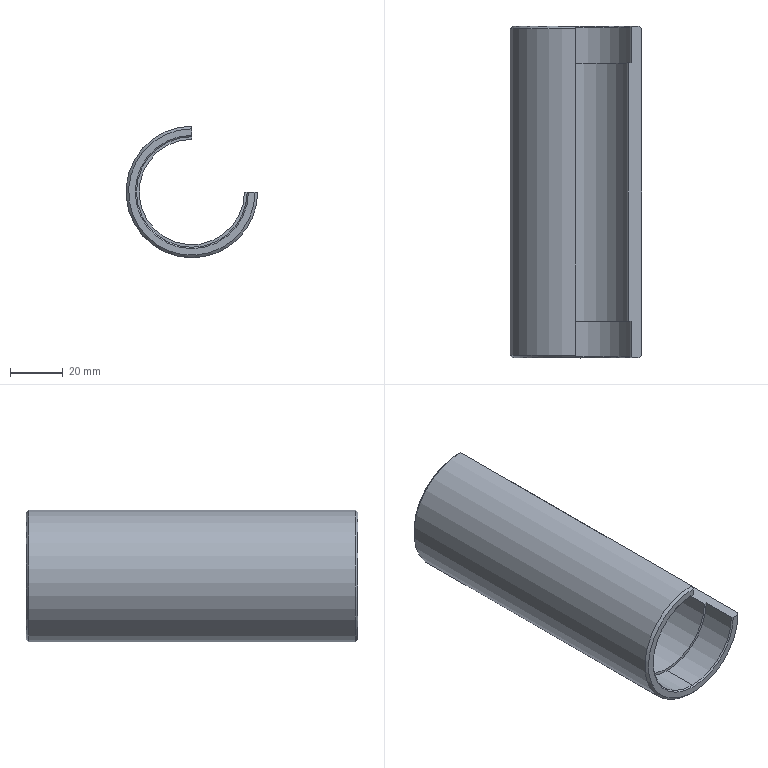Part | STEP file | 1 solid | 18 faces | box 50 x 126 x 50 mm | volume 63952 mm3 | cone 6 | cylinder 6 | plane 6 | commonest cylinder face diameters 42 x3 50 x2 40 x1
STEP:
#1=CARTESIAN_POINT('',(0.,0.,0.));
#2=DIRECTION('',(0.,0.,1.));
#3=DIRECTION('',(1.,0.,0.));
#4=AXIS2_PLACEMENT_3D('',#1,#2,#3);
#5=CARTESIAN_POINT('',(0.,63.,-24.));
#6=VERTEX_POINT('',#5);
#7=CARTESIAN_POINT('',(0.,63.,24.));
#8=VERTEX_POINT('',#7);
#9=CARTESIAN_POINT('',(0.,63.,0.));
#10=DIRECTION('',(0.,1.,0.));
#11=DIRECTION('',(0.,0.,1.));
#12=AXIS2_PLACEMENT_3D('',#9,#10,#11);
#13=CIRCLE('',#12,24.);
#14=CARTESIAN_POINT('',(0.,63.,0.));
#15=DIRECTION('',(0.,-1.,0.));
#16=DIRECTION('',(0.,0.,-1.));
#17=AXIS2_PLACEMENT_3D('',#14,#15,#16);
#18=CONICAL_SURFACE('',#17,24.,0.7854);
#19=CARTESIAN_POINT('',(9.425,0.));
#20=DIRECTION('',(-1.,0.));
#21=VECTOR('',#20,1.);
#22=LINE('',#19,#21);
#23=(GEOMETRIC_REPRESENTATION_CONTEXT(2)PARAMETRIC_REPRESENTATION_CONTEXT()REPRESENTATION_CONTEXT('',''));
#24=DEFINITIONAL_REPRESENTATION('',(#22),#23);
#25=PCURVE('',#18,#24);
#26=CARTESIAN_POINT('',(0.,63.,0.));
#27=DIRECTION('',(0.,1.,0.));
#28=DIRECTION('',(0.,0.,1.));
#29=AXIS2_PLACEMENT_3D('',#26,#27,#28);
#30=PLANE('',#29);
#31=CARTESIAN_POINT('',(0.,0.));
#32=DIRECTION('',(1.,0.));
#33=AXIS2_PLACEMENT_2D('',#31,#32);
#34=CIRCLE('',#33,24.);
#35=(GEOMETRIC_REPRESENTATION_CONTEXT(2)PARAMETRIC_REPRESENTATION_CONTEXT()REPRESENTATION_CONTEXT('',''));
#36=DEFINITIONAL_REPRESENTATION('',(#34),#35);
#37=PCURVE('',#30,#36);
#38=SURFACE_CURVE('',#13,(#25,#37),.PCURVE_S1.);
#39=EDGE_CURVE('',#6,#8,#38,.T.);
#40=ORIENTED_EDGE('',*,*,#39,.F.);
#41=CARTESIAN_POINT('',(0.,62.,-25.));
#42=VERTEX_POINT('',#41);
#43=CARTESIAN_POINT('',(0.,63.,-24.));
#44=DIRECTION('',(0.,-0.7071,-0.7071));
#45=VECTOR('',#44,1.);
#46=LINE('',#43,#45);
#47=CARTESIAN_POINT('',(6.283,0.));
#48=DIRECTION('',(0.,1.));
#49=VECTOR('',#48,1.);
#50=LINE('',#47,#49);
#51=(GEOMETRIC_REPRESENTATION_CONTEXT(2)PARAMETRIC_REPRESENTATION_CONTEXT()REPRESENTATION_CONTEXT('',''));
#52=DEFINITIONAL_REPRESENTATION('',(#50),#51);
#53=PCURVE('',#18,#52);
#54=CARTESIAN_POINT('',(0.,63.,0.));
#55=DIRECTION('',(0.,-1.,0.));
#56=DIRECTION('',(0.,0.,-1.));
#57=AXIS2_PLACEMENT_3D('',#54,#55,#56);
#58=CONICAL_SURFACE('',#57,24.,0.7854);
#59=CARTESIAN_POINT('',(0.,0.));
#60=DIRECTION('',(0.,1.));
#61=VECTOR('',#60,1.);
#62=LINE('',#59,#61);
#63=(GEOMETRIC_REPRESENTATION_CONTEXT(2)PARAMETRIC_REPRESENTATION_CONTEXT()REPRESENTATION_CONTEXT('',''));
#64=DEFINITIONAL_REPRESENTATION('',(#62),#63);
#65=PCURVE('',#58,#64);
#66=SURFACE_CURVE('',#46,(#53,#65),.PCURVE_S1.);
#67=EDGE_CURVE('',#6,#42,#66,.T.);
#68=ORIENTED_EDGE('',*,*,#67,.T.);
#69=CARTESIAN_POINT('',(0.,62.,25.));
#70=VERTEX_POINT('',#69);
#71=CARTESIAN_POINT('',(0.,62.,0.));
#72=DIRECTION('',(0.,-1.,0.));
#73=DIRECTION('',(0.,0.,1.));
#74=AXIS2_PLACEMENT_3D('',#71,#72,#73);
#75=CIRCLE('',#74,25.);
#76=CARTESIAN_POINT('',(3.142,1.));
#77=DIRECTION('',(1.,0.));
#78=VECTOR('',#77,1.);
#79=LINE('',#76,#78);
#80=(GEOMETRIC_REPRESENTATION_CONTEXT(2)PARAMETRIC_REPRESENTATION_CONTEXT()REPRESENTATION_CONTEXT('',''));
#81=DEFINITIONAL_REPRESENTATION('',(#79),#80);
#82=PCURVE('',#18,#81);
#83=CARTESIAN_POINT('',(0.,63.,0.));
#84=DIRECTION('',(0.,-1.,0.));
#85=DIRECTION('',(0.,0.,-1.));
#86=AXIS2_PLACEMENT_3D('',#83,#84,#85);
#87=CYLINDRICAL_SURFACE('',#86,25.);
#88=CARTESIAN_POINT('',(3.142,1.));
#89=DIRECTION('',(1.,0.));
#90=VECTOR('',#89,1.);
#91=LINE('',#88,#90);
#92=(GEOMETRIC_REPRESENTATION_CONTEXT(2)PARAMETRIC_REPRESENTATION_CONTEXT()REPRESENTATION_CONTEXT('',''));
#93=DEFINITIONAL_REPRESENTATION('',(#91),#92);
#94=PCURVE('',#87,#93);
#95=SURFACE_CURVE('',#75,(#82,#94),.PCURVE_S1.);
#96=EDGE_CURVE('',#70,#42,#95,.T.);
#97=ORIENTED_EDGE('',*,*,#96,.F.);
#98=CARTESIAN_POINT('',(0.,87.,0.));
#99=DIRECTION('',(0.,-0.7071,0.7071));
#100=VECTOR('',#99,1.);
#101=LINE('',#98,#100);
#102=CARTESIAN_POINT('',(3.142,-24.));
#103=DIRECTION('',(0.,1.));
#104=VECTOR('',#103,1.);
#105=LINE('',#102,#104);
#106=(GEOMETRIC_REPRESENTATION_CONTEXT(2)PARAMETRIC_REPRESENTATION_CONTEXT()REPRESENTATION_CONTEXT('',''));
#107=DEFINITIONAL_REPRESENTATION('',(#105),#106);
#108=PCURVE('',#18,#107);
#109=CARTESIAN_POINT('',(0.,95.,25.));
#110=DIRECTION('',(-1.,0.,0.));
#111=DIRECTION('',(0.,0.,1.));
#112=AXIS2_PLACEMENT_3D('',#109,#110,#111);
#113=PLANE('',#112);
#114=CARTESIAN_POINT('',(-25.,-8.));
#115=DIRECTION('',(0.7071,-0.7071));
#116=VECTOR('',#115,1.);
#117=LINE('',#114,#116);
#118=(GEOMETRIC_REPRESENTATION_CONTEXT(2)PARAMETRIC_REPRESENTATION_CONTEXT()REPRESENTATION_CONTEXT('',''));
#119=DEFINITIONAL_REPRESENTATION('',(#117),#118);
#120=PCURVE('',#113,#119);
#121=SURFACE_CURVE('',#101,(#108,#120),.PCURVE_S1.);
#122=EDGE_CURVE('',#8,#70,#121,.T.);
#123=ORIENTED_EDGE('',*,*,#122,.F.);
#124=EDGE_LOOP('',(#40,#68,#97,#123));
#125=FACE_BOUND('',#124,.T.);
#126=ADVANCED_FACE('',(#125),#18,.T.);
#127=CARTESIAN_POINT('',(21.,-62.5,0.));
#128=VERTEX_POINT('',#127);
#129=CARTESIAN_POINT('',(21.5,-63.,0.));
#130=VERTEX_POINT('',#129);
#131=CARTESIAN_POINT('',(0.,-41.5,0.));
#132=DIRECTION('',(0.7071,-0.7071,0.));
#133=VECTOR('',#132,1.);
#134=LINE('',#131,#133);
#135=CARTESIAN_POINT('',(0.,-63.,0.));
#136=DIRECTION('',(0.,-1.,0.));
#137=DIRECTION('',(0.,0.,-1.));
#138=AXIS2_PLACEMENT_3D('',#135,#136,#137);
#139=CONICAL_SURFACE('',#138,21.5,0.7854);
#140=CARTESIAN_POINT('',(1.571,-21.5));
#141=DIRECTION('',(0.,1.));
#142=VECTOR('',#141,1.);
#143=LINE('',#140,#142);
#144=(GEOMETRIC_REPRESENTATION_CONTEXT(2)PARAMETRIC_REPRESENTATION_CONTEXT()REPRESENTATION_CONTEXT('',''));
#145=DEFINITIONAL_REPRESENTATION('',(#143),#144);
#146=PCURVE('',#139,#145);
#147=CARTESIAN_POINT('',(0.,95.,0.));
#148=DIRECTION('',(0.,0.,-1.));
#149=DIRECTION('',(-1.,0.,0.));
#150=AXIS2_PLACEMENT_3D('',#147,#148,#149);
#151=PLANE('',#150);
#152=CARTESIAN_POINT('',(0.,-136.5));
#153=DIRECTION('',(-0.7071,-0.7071));
#154=VECTOR('',#153,1.);
#155=LINE('',#152,#154);
#156=(GEOMETRIC_REPRESENTATION_CONTEXT(2)PARAMETRIC_REPRESENTATION_CONTEXT()REPRESENTATION_CONTEXT('',''));
#157=DEFINITIONAL_REPRESENTATION('',(#155),#156);
#158=PCURVE('',#151,#157);
#159=SURFACE_CURVE('',#134,(#146,#158),.PCURVE_S1.);
#160=EDGE_CURVE('',#128,#130,#159,.T.);
#161=ORIENTED_EDGE('',*,*,#160,.T.);
#162=CARTESIAN_POINT('',(0.,-63.,-21.5));
#163=VERTEX_POINT('',#162);
#164=CARTESIAN_POINT('',(0.,-63.,0.));
#165=DIRECTION('',(0.,1.,0.));
#166=DIRECTION('',(0.,0.,1.));
#167=AXIS2_PLACEMENT_3D('',#164,#165,#166);
#168=CIRCLE('',#167,21.5);
#169=CARTESIAN_POINT('',(3.142,0.));
#170=DIRECTION('',(-1.,0.));
#171=VECTOR('',#170,1.);
#172=LINE('',#169,#171);
#173=(GEOMETRIC_REPRESENTATION_CONTEXT(2)PARAMETRIC_REPRESENTATION_CONTEXT()REPRESENTATION_CONTEXT('',''));
#174=DEFINITIONAL_REPRESENTATION('',(#172),#173);
#175=PCURVE('',#139,#174);
#176=CARTESIAN_POINT('',(0.,-63.,0.));
#177=DIRECTION('',(0.,1.,0.));
#178=DIRECTION('',(0.,0.,1.));
#179=AXIS2_PLACEMENT_3D('',#176,#177,#178);
#180=PLANE('',#179);
#181=CARTESIAN_POINT('',(0.,0.));
#182=DIRECTION('',(1.,0.));
#183=AXIS2_PLACEMENT_2D('',#181,#182);
#184=CIRCLE('',#183,21.5);
#185=(GEOMETRIC_REPRESENTATION_CONTEXT(2)PARAMETRIC_REPRESENTATION_CONTEXT()REPRESENTATION_CONTEXT('',''));
#186=DEFINITIONAL_REPRESENTATION('',(#184),#185);
#187=PCURVE('',#180,#186);
#188=SURFACE_CURVE('',#168,(#175,#187),.PCURVE_S1.);
#189=EDGE_CURVE('',#130,#163,#188,.T.);
#190=ORIENTED_EDGE('',*,*,#189,.T.);
#191=CARTESIAN_POINT('',(0.,-62.5,-21.));
#192=VERTEX_POINT('',#191);
#193=CARTESIAN_POINT('',(0.,-63.,-21.5));
#194=DIRECTION('',(0.,-0.7071,-0.7071));
#195=VECTOR('',#194,1.);
#196=LINE('',#193,#195);
#197=CARTESIAN_POINT('',(0.,0.));
#198=DIRECTION('',(0.,1.));
#199=VECTOR('',#198,1.);
#200=LINE('',#197,#199);
#201=(GEOMETRIC_REPRESENTATION_CONTEXT(2)PARAMETRIC_REPRESENTATION_CONTEXT()REPRESENTATION_CONTEXT('',''));
#202=DEFINITIONAL_REPRESENTATION('',(#200),#201);
#203=PCURVE('',#139,#202);
#204=CARTESIAN_POINT('',(0.,-63.,0.));
#205=DIRECTION('',(0.,-1.,0.));
#206=DIRECTION('',(0.,0.,-1.));
#207=AXIS2_PLACEMENT_3D('',#204,#205,#206);
#208=CONICAL_SURFACE('',#207,21.5,0.7854);
#209=CARTESIAN_POINT('',(6.283,0.));
#210=DIRECTION('',(0.,1.));
#211=VECTOR('',#210,1.);
#212=LINE('',#209,#211);
#213=(GEOMETRIC_REPRESENTATION_CONTEXT(2)PARAMETRIC_REPRESENTATION_CONTEXT()REPRESENTATION_CONTEXT('',''));
#214=DEFINITIONAL_REPRESENTATION('',(#212),#213);
#215=PCURVE('',#208,#214);
#216=SURFACE_CURVE('',#196,(#203,#215),.PCURVE_S1.);
#217=EDGE_CURVE('',#192,#163,#216,.T.);
#218=ORIENTED_EDGE('',*,*,#217,.F.);
#219=CARTESIAN_POINT('',(0.,-62.5,0.));
#220=DIRECTION('',(0.,-1.,0.));
#221=DIRECTION('',(0.,0.,1.));
#222=AXIS2_PLACEMENT_3D('',#219,#220,#221);
#223=CIRCLE('',#222,21.);
#224=CARTESIAN_POINT('',(-3.142,-0.5));
#225=DIRECTION('',(1.,0.));
#226=VECTOR('',#225,1.);
#227=LINE('',#224,#226);
#228=(GEOMETRIC_REPRESENTATION_CONTEXT(2)PARAMETRIC_REPRESENTATION_CONTEXT()REPRESENTATION_CONTEXT('',''));
#229=DEFINITIONAL_REPRESENTATION('',(#227),#228);
#230=PCURVE('',#139,#229);
#231=CARTESIAN_POINT('',(0.,-49.,0.));
#232=DIRECTION('',(0.,-1.,0.));
#233=DIRECTION('',(0.,0.,-1.));
#234=AXIS2_PLACEMENT_3D('',#231,#232,#233);
#235=CYLINDRICAL_SURFACE('',#234,21.);
#236=CARTESIAN_POINT('',(-3.142,13.5));
#237=DIRECTION('',(1.,0.));
#238=VECTOR('',#237,1.);
#239=LINE('',#236,#238);
#240=(GEOMETRIC_REPRESENTATION_CONTEXT(2)PARAMETRIC_REPRESENTATION_CONTEXT()REPRESENTATION_CONTEXT('',''));
#241=DEFINITIONAL_REPRESENTATION('',(#239),#240);
#242=PCURVE('',#235,#241);
#243=SURFACE_CURVE('',#223,(#230,#242),.PCURVE_S1.);
#244=EDGE_CURVE('',#192,#128,#243,.T.);
#245=ORIENTED_EDGE('',*,*,#244,.T.);
#246=EDGE_LOOP('',(#161,#190,#218,#245));
#247=FACE_BOUND('',#246,.F.);
#248=ADVANCED_FACE('',(#247),#139,.F.);
#249=CARTESIAN_POINT('',(21.,-49.,0.));
#250=VERTEX_POINT('',#249);
#251=CARTESIAN_POINT('',(21.,-49.,0.));
#252=DIRECTION('',(0.,-1.,0.));
#253=VECTOR('',#252,1.);
#254=LINE('',#251,#253);
#255=CARTESIAN_POINT('',(1.571,0.));
#256=DIRECTION('',(0.,1.));
#257=VECTOR('',#256,1.);
#258=LINE('',#255,#257);
#259=(GEOMETRIC_REPRESENTATION_CONTEXT(2)PARAMETRIC_REPRESENTATION_CONTEXT()REPRESENTATION_CONTEXT('',''));
#260=DEFINITIONAL_REPRESENTATION('',(#258),#259);
#261=PCURVE('',#235,#260);
#262=CARTESIAN_POINT('',(-21.,-144.));
#263=DIRECTION('',(0.,-1.));
#264=VECTOR('',#263,1.);
#265=LINE('',#262,#264);
#266=(GEOMETRIC_REPRESENTATION_CONTEXT(2)PARAMETRIC_REPRESENTATION_CONTEXT()REPRESENTATION_CONTEXT('',''));
#267=DEFINITIONAL_REPRESENTATION('',(#265),#266);
#268=PCURVE('',#151,#267);
#269=SURFACE_CURVE('',#254,(#261,#268),.PCURVE_S1.);
#270=EDGE_CURVE('',#250,#128,#269,.T.);
#271=ORIENTED_EDGE('',*,*,#270,.T.);
#272=ORIENTED_EDGE('',*,*,#244,.F.);
#273=CARTESIAN_POINT('',(0.,-49.,-21.));
#274=VERTEX_POINT('',#273);
#275=CARTESIAN_POINT('',(0.,-49.,-21.));
#276=DIRECTION('',(0.,-1.,0.));
#277=VECTOR('',#276,1.);
#278=LINE('',#275,#277);
#279=CARTESIAN_POINT('',(0.,0.));
#280=DIRECTION('',(0.,1.));
#281=VECTOR('',#280,1.);
#282=LINE('',#279,#281);
#283=(GEOMETRIC_REPRESENTATION_CONTEXT(2)PARAMETRIC_REPRESENTATION_CONTEXT()REPRESENTATION_CONTEXT('',''));
#284=DEFINITIONAL_REPRESENTATION('',(#282),#283);
#285=PCURVE('',#235,#284);
#286=CARTESIAN_POINT('',(0.,-49.,0.));
#287=DIRECTION('',(0.,-1.,0.));
#288=DIRECTION('',(0.,0.,-1.));
#289=AXIS2_PLACEMENT_3D('',#286,#287,#288);
#290=CYLINDRICAL_SURFACE('',#289,21.);
#291=CARTESIAN_POINT('',(6.283,0.));
#292=DIRECTION('',(0.,1.));
#293=VECTOR('',#292,1.);
#294=LINE('',#291,#293);
#295=(GEOMETRIC_REPRESENTATION_CONTEXT(2)PARAMETRIC_REPRESENTATION_CONTEXT()REPRESENTATION_CONTEXT('',''));
#296=DEFINITIONAL_REPRESENTATION('',(#294),#295);
#297=PCURVE('',#290,#296);
#298=SURFACE_CURVE('',#278,(#285,#297),.PCURVE_S1.);
#299=EDGE_CURVE('',#274,#192,#298,.T.);
#300=ORIENTED_EDGE('',*,*,#299,.F.);
#301=CARTESIAN_POINT('',(0.,-49.,0.));
#302=DIRECTION('',(0.,1.,0.));
#303=DIRECTION('',(0.,0.,1.));
#304=AXIS2_PLACEMENT_3D('',#301,#302,#303);
#305=CIRCLE('',#304,21.);
#306=CARTESIAN_POINT('',(3.142,0.));
#307=DIRECTION('',(-1.,0.));
#308=VECTOR('',#307,1.);
#309=LINE('',#306,#308);
#310=(GEOMETRIC_REPRESENTATION_CONTEXT(2)PARAMETRIC_REPRESENTATION_CONTEXT()REPRESENTATION_CONTEXT('',''));
#311=DEFINITIONAL_REPRESENTATION('',(#309),#310);
#312=PCURVE('',#235,#311);
#313=CARTESIAN_POINT('',(0.,-49.,0.));
#314=DIRECTION('',(0.,-1.,0.));
#315=DIRECTION('',(0.,0.,1.));
#316=AXIS2_PLACEMENT_3D('',#313,#314,#315);
#317=PLANE('',#316);
#318=CARTESIAN_POINT('',(21.,0.));
#319=CARTESIAN_POINT('',(21.,-36.373));
#320=CARTESIAN_POINT('',(-10.5,-18.187));
#321=CARTESIAN_POINT('',(-42.,0.));
#322=CARTESIAN_POINT('',(-10.5,18.187));
#323=CARTESIAN_POINT('',(21.,36.373));
#324=CARTESIAN_POINT('',(21.,0.));
#325=(BOUNDED_CURVE()B_SPLINE_CURVE(2,(#318,#319,#320,#321,#322,#323,#324),.UNSPECIFIED.,.T.,.F.)B_SPLINE_CURVE_WITH_KNOTS((1,2,2,2,2,1),(-2.094,0.,2.094,4.189,6.283,8.378),.UNSPECIFIED.)CURVE()GEOMETRIC_REPRESENTATION_ITEM()RATIONAL_B_SPLINE_CURVE((1.,0.5,1.,0.5,1.,0.5,1.))REPRESENTATION_ITEM(''));
#326=(GEOMETRIC_REPRESENTATION_CONTEXT(2)PARAMETRIC_REPRESENTATION_CONTEXT()REPRESENTATION_CONTEXT('',''));
#327=DEFINITIONAL_REPRESENTATION('',(#325),#326);
#328=PCURVE('',#317,#327);
#329=SURFACE_CURVE('',#305,(#312,#328),.PCURVE_S1.);
#330=EDGE_CURVE('',#250,#274,#329,.T.);
#331=ORIENTED_EDGE('',*,*,#330,.F.);
#332=EDGE_LOOP('',(#271,#272,#300,#331));
#333=FACE_BOUND('',#332,.F.);
#334=ADVANCED_FACE('',(#333),#235,.F.);
#335=ORIENTED_EDGE('',*,*,#96,.T.);
#336=CARTESIAN_POINT('',(0.,-62.,-25.));
#337=VERTEX_POINT('',#336);
#338=CARTESIAN_POINT('',(0.,63.,-25.));
#339=DIRECTION('',(0.,-1.,0.));
#340=VECTOR('',#339,1.);
#341=LINE('',#338,#340);
#342=CARTESIAN_POINT('',(6.283,0.));
#343=DIRECTION('',(0.,1.));
#344=VECTOR('',#343,1.);
#345=LINE('',#342,#344);
#346=(GEOMETRIC_REPRESENTATION_CONTEXT(2)PARAMETRIC_REPRESENTATION_CONTEXT()REPRESENTATION_CONTEXT('',''));
#347=DEFINITIONAL_REPRESENTATION('',(#345),#346);
#348=PCURVE('',#87,#347);
#349=CARTESIAN_POINT('',(0.,63.,0.));
#350=DIRECTION('',(0.,-1.,0.));
#351=DIRECTION('',(0.,0.,-1.));
#352=AXIS2_PLACEMENT_3D('',#349,#350,#351);
#353=CYLINDRICAL_SURFACE('',#352,25.);
#354=CARTESIAN_POINT('',(0.,0.));
#355=DIRECTION('',(0.,1.));
#356=VECTOR('',#355,1.);
#357=LINE('',#354,#356);
#358=(GEOMETRIC_REPRESENTATION_CONTEXT(2)PARAMETRIC_REPRESENTATION_CONTEXT()REPRESENTATION_CONTEXT('',''));
#359=DEFINITIONAL_REPRESENTATION('',(#357),#358);
#360=PCURVE('',#353,#359);
#361=SURFACE_CURVE('',#341,(#348,#360),.PCURVE_S1.);
#362=EDGE_CURVE('',#42,#337,#361,.T.);
#363=ORIENTED_EDGE('',*,*,#362,.T.);
#364=CARTESIAN_POINT('',(0.,-62.,25.));
#365=VERTEX_POINT('',#364);
#366=CARTESIAN_POINT('',(0.,-62.,0.));
#367=DIRECTION('',(0.,1.,0.));
#368=DIRECTION('',(0.,0.,1.));
#369=AXIS2_PLACEMENT_3D('',#366,#367,#368);
#370=CIRCLE('',#369,25.);
#371=CARTESIAN_POINT('',(9.425,125.));
#372=DIRECTION('',(-1.,0.));
#373=VECTOR('',#372,1.);
#374=LINE('',#371,#373);
#375=(GEOMETRIC_REPRESENTATION_CONTEXT(2)PARAMETRIC_REPRESENTATION_CONTEXT()REPRESENTATION_CONTEXT('',''));
#376=DEFINITIONAL_REPRESENTATION('',(#374),#375);
#377=PCURVE('',#87,#376);
#378=CARTESIAN_POINT('',(0.,-62.,0.));
#379=DIRECTION('',(0.,1.,0.));
#380=DIRECTION('',(0.,0.,1.));
#381=AXIS2_PLACEMENT_3D('',#378,#379,#380);
#382=CONICAL_SURFACE('',#381,25.,0.7854);
#383=CARTESIAN_POINT('',(0.,0.));
#384=DIRECTION('',(1.,0.));
#385=VECTOR('',#384,1.);
#386=LINE('',#383,#385);
#387=(GEOMETRIC_REPRESENTATION_CONTEXT(2)PARAMETRIC_REPRESENTATION_CONTEXT()REPRESENTATION_CONTEXT('',''));
#388=DEFINITIONAL_REPRESENTATION('',(#386),#387);
#389=PCURVE('',#382,#388);
#390=SURFACE_CURVE('',#370,(#377,#389),.PCURVE_S1.);
#391=EDGE_CURVE('',#337,#365,#390,.T.);
#392=ORIENTED_EDGE('',*,*,#391,.T.);
#393=CARTESIAN_POINT('',(0.,95.,25.));
#394=DIRECTION('',(0.,-1.,0.));
#395=VECTOR('',#394,1.);
#396=LINE('',#393,#395);
#397=CARTESIAN_POINT('',(3.142,-32.));
#398=DIRECTION('',(0.,1.));
#399=VECTOR('',#398,1.);
#400=LINE('',#397,#399);
#401=(GEOMETRIC_REPRESENTATION_CONTEXT(2)PARAMETRIC_REPRESENTATION_CONTEXT()REPRESENTATION_CONTEXT('',''));
#402=DEFINITIONAL_REPRESENTATION('',(#400),#401);
#403=PCURVE('',#87,#402);
#404=CARTESIAN_POINT('',(0.,0.));
#405=DIRECTION('',(0.,-1.));
#406=VECTOR('',#405,1.);
#407=LINE('',#404,#406);
#408=(GEOMETRIC_REPRESENTATION_CONTEXT(2)PARAMETRIC_REPRESENTATION_CONTEXT()REPRESENTATION_CONTEXT('',''));
#409=DEFINITIONAL_REPRESENTATION('',(#407),#408);
#410=PCURVE('',#113,#409);
#411=SURFACE_CURVE('',#396,(#403,#410),.PCURVE_S1.);
#412=EDGE_CURVE('',#70,#365,#411,.T.);
#413=ORIENTED_EDGE('',*,*,#412,.F.);
#414=EDGE_LOOP('',(#335,#363,#392,#413));
#415=FACE_BOUND('',#414,.T.);
#416=ADVANCED_FACE('',(#415),#87,.T.);
#417=ORIENTED_EDGE('',*,*,#362,.F.);
#418=CARTESIAN_POINT('',(25.,62.,0.));
#419=VERTEX_POINT('',#418);
#420=CARTESIAN_POINT('',(0.,62.,0.));
#421=DIRECTION('',(0.,-1.,0.));
#422=DIRECTION('',(0.,0.,1.));
#423=AXIS2_PLACEMENT_3D('',#420,#421,#422);
#424=CIRCLE('',#423,25.);
#425=CARTESIAN_POINT('',(-3.142,1.));
#426=DIRECTION('',(1.,0.));
#427=VECTOR('',#426,1.);
#428=LINE('',#425,#427);
#429=(GEOMETRIC_REPRESENTATION_CONTEXT(2)PARAMETRIC_REPRESENTATION_CONTEXT()REPRESENTATION_CONTEXT('',''));
#430=DEFINITIONAL_REPRESENTATION('',(#428),#429);
#431=PCURVE('',#353,#430);
#432=CARTESIAN_POINT('',(-3.142,1.));
#433=DIRECTION('',(1.,0.));
#434=VECTOR('',#433,1.);
#435=LINE('',#432,#434);
#436=(GEOMETRIC_REPRESENTATION_CONTEXT(2)PARAMETRIC_REPRESENTATION_CONTEXT()REPRESENTATION_CONTEXT('',''));
#437=DEFINITIONAL_REPRESENTATION('',(#435),#436);
#438=PCURVE('',#58,#437);
#439=SURFACE_CURVE('',#424,(#431,#438),.PCURVE_S1.);
#440=EDGE_CURVE('',#42,#419,#439,.T.);
#441=ORIENTED_EDGE('',*,*,#440,.T.);
#442=CARTESIAN_POINT('',(25.,-62.,0.));
#443=VERTEX_POINT('',#442);
#444=CARTESIAN_POINT('',(25.,63.,0.));
#445=DIRECTION('',(0.,-1.,0.));
#446=VECTOR('',#445,1.);
#447=LINE('',#444,#446);
#448=CARTESIAN_POINT('',(1.571,0.));
#449=DIRECTION('',(0.,1.));
#450=VECTOR('',#449,1.);
#451=LINE('',#448,#450);
#452=(GEOMETRIC_REPRESENTATION_CONTEXT(2)PARAMETRIC_REPRESENTATION_CONTEXT()REPRESENTATION_CONTEXT('',''));
#453=DEFINITIONAL_REPRESENTATION('',(#451),#452);
#454=PCURVE('',#353,#453);
#455=CARTESIAN_POINT('',(-25.,-32.));
#456=DIRECTION('',(0.,-1.));
#457=VECTOR('',#456,1.);
#458=LINE('',#455,#457);
#459=(GEOMETRIC_REPRESENTATION_CONTEXT(2)PARAMETRIC_REPRESENTATION_CONTEXT()REPRESENTATION_CONTEXT('',''));
#460=DEFINITIONAL_REPRESENTATION('',(#458),#459);
#461=PCURVE('',#151,#460);
#462=SURFACE_CURVE('',#447,(#454,#461),.PCURVE_S1.);
#463=EDGE_CURVE('',#419,#443,#462,.T.);
#464=ORIENTED_EDGE('',*,*,#463,.T.);
#465=CARTESIAN_POINT('',(0.,-62.,0.));
#466=DIRECTION('',(0.,1.,0.));
#467=DIRECTION('',(0.,0.,1.));
#468=AXIS2_PLACEMENT_3D('',#465,#466,#467);
#469=CIRCLE('',#468,25.);
#470=CARTESIAN_POINT('',(3.142,125.));
#471=DIRECTION('',(-1.,0.));
#472=VECTOR('',#471,1.);
#473=LINE('',#470,#472);
#474=(GEOMETRIC_REPRESENTATION_CONTEXT(2)PARAMETRIC_REPRESENTATION_CONTEXT()REPRESENTATION_CONTEXT('',''));
#475=DEFINITIONAL_REPRESENTATION('',(#473),#474);
#476=PCURVE('',#353,#475);
#477=CARTESIAN_POINT('',(0.,0.));
#478=DIRECTION('',(1.,0.));
#479=VECTOR('',#478,1.);
#480=LINE('',#477,#479);
#481=(GEOMETRIC_REPRESENTATION_CONTEXT(2)PARAMETRIC_REPRESENTATION_CONTEXT()REPRESENTATION_CONTEXT('',''));
#482=DEFINITIONAL_REPRESENTATION('',(#480),#481);
#483=PCURVE('',#382,#482);
#484=SURFACE_CURVE('',#469,(#476,#483),.PCURVE_S1.);
#485=EDGE_CURVE('',#443,#337,#484,.T.);
#486=ORIENTED_EDGE('',*,*,#485,.T.);
#487=EDGE_LOOP('',(#417,#441,#464,#486));
#488=FACE_BOUND('',#487,.T.);
#489=ADVANCED_FACE('',(#488),#353,.T.);
#490=ORIENTED_EDGE('',*,*,#189,.T.);
#491=CARTESIAN_POINT('',(0.,-63.,21.5));
#492=VERTEX_POINT('',#491);
#493=CARTESIAN_POINT('',(0.,-63.,0.));
#494=DIRECTION('',(0.,1.,0.));
#495=DIRECTION('',(0.,0.,1.));
#496=AXIS2_PLACEMENT_3D('',#493,#494,#495);
#497=CIRCLE('',#496,21.5);
#498=CARTESIAN_POINT('',(0.,0.));
#499=DIRECTION('',(1.,0.));
#500=AXIS2_PLACEMENT_2D('',#498,#499);
#501=CIRCLE('',#500,21.5);
#502=(GEOMETRIC_REPRESENTATION_CONTEXT(2)PARAMETRIC_REPRESENTATION_CONTEXT()REPRESENTATION_CONTEXT('',''));
#503=DEFINITIONAL_REPRESENTATION('',(#501),#502);
#504=PCURVE('',#180,#503);
#505=CARTESIAN_POINT('',(9.425,0.));
#506=DIRECTION('',(-1.,0.));
#507=VECTOR('',#506,1.);
#508=LINE('',#505,#507);
#509=(GEOMETRIC_REPRESENTATION_CONTEXT(2)PARAMETRIC_REPRESENTATION_CONTEXT()REPRESENTATION_CONTEXT('',''));
#510=DEFINITIONAL_REPRESENTATION('',(#508),#509);
#511=PCURVE('',#208,#510);
#512=SURFACE_CURVE('',#497,(#504,#511),.PCURVE_S1.);
#513=EDGE_CURVE('',#163,#492,#512,.T.);
#514=ORIENTED_EDGE('',*,*,#513,.T.);
#515=CARTESIAN_POINT('',(0.,-63.,24.));
#516=VERTEX_POINT('',#515);
#517=CARTESIAN_POINT('',(0.,-63.,0.));
#518=DIRECTION('',(0.,0.,1.));
#519=VECTOR('',#518,1.);
#520=LINE('',#517,#519);
#521=CARTESIAN_POINT('',(0.,0.));
#522=DIRECTION('',(1.,0.));
#523=VECTOR('',#522,1.);
#524=LINE('',#521,#523);
#525=(GEOMETRIC_REPRESENTATION_CONTEXT(2)PARAMETRIC_REPRESENTATION_CONTEXT()REPRESENTATION_CONTEXT('',''));
#526=DEFINITIONAL_REPRESENTATION('',(#524),#525);
#527=PCURVE('',#180,#526);
#528=CARTESIAN_POINT('',(-25.,-158.));
#529=DIRECTION('',(1.,0.));
#530=VECTOR('',#529,1.);
#531=LINE('',#528,#530);
#532=(GEOMETRIC_REPRESENTATION_CONTEXT(2)PARAMETRIC_REPRESENTATION_CONTEXT()REPRESENTATION_CONTEXT('',''));
#533=DEFINITIONAL_REPRESENTATION('',(#531),#532);
#534=PCURVE('',#113,#533);
#535=SURFACE_CURVE('',#520,(#527,#534),.PCURVE_S1.);
#536=EDGE_CURVE('',#492,#516,#535,.T.);
#537=ORIENTED_EDGE('',*,*,#536,.T.);
#538=CARTESIAN_POINT('',(24.,-63.,0.));
#539=VERTEX_POINT('',#538);
#540=CARTESIAN_POINT('',(0.,-63.,0.));
#541=DIRECTION('',(0.,-1.,0.));
#542=DIRECTION('',(0.,0.,1.));
#543=AXIS2_PLACEMENT_3D('',#540,#541,#542);
#544=CIRCLE('',#543,24.);
#545=CARTESIAN_POINT('',(24.,0.));
#546=CARTESIAN_POINT('',(24.,-41.569));
#547=CARTESIAN_POINT('',(-12.,-20.785));
#548=CARTESIAN_POINT('',(-48.,0.));
#549=CARTESIAN_POINT('',(-12.,20.785));
#550=CARTESIAN_POINT('',(24.,41.569));
#551=CARTESIAN_POINT('',(24.,0.));
#552=(BOUNDED_CURVE()B_SPLINE_CURVE(2,(#545,#546,#547,#548,#549,#550,#551),.UNSPECIFIED.,.T.,.F.)B_SPLINE_CURVE_WITH_KNOTS((1,2,2,2,2,1),(-2.094,0.,2.094,4.189,6.283,8.378),.UNSPECIFIED.)CURVE()GEOMETRIC_REPRESENTATION_ITEM()RATIONAL_B_SPLINE_CURVE((1.,0.5,1.,0.5,1.,0.5,1.))REPRESENTATION_ITEM(''));
#553=(GEOMETRIC_REPRESENTATION_CONTEXT(2)PARAMETRIC_REPRESENTATION_CONTEXT()REPRESENTATION_CONTEXT('',''));
#554=DEFINITIONAL_REPRESENTATION('',(#552),#553);
#555=PCURVE('',#180,#554);
#556=CARTESIAN_POINT('',(6.283,-1.));
#557=DIRECTION('',(-1.,0.));
#558=VECTOR('',#557,1.);
#559=LINE('',#556,#558);
#560=(GEOMETRIC_REPRESENTATION_CONTEXT(2)PARAMETRIC_REPRESENTATION_CONTEXT()REPRESENTATION_CONTEXT('',''));
#561=DEFINITIONAL_REPRESENTATION('',(#559),#560);
#562=PCURVE('',#382,#561);
#563=SURFACE_CURVE('',#544,(#555,#562),.PCURVE_S1.);
#564=EDGE_CURVE('',#516,#539,#563,.T.);
#565=ORIENTED_EDGE('',*,*,#564,.T.);
#566=CARTESIAN_POINT('',(0.,-63.,0.));
#567=DIRECTION('',(-1.,0.,0.));
#568=VECTOR('',#567,1.);
#569=LINE('',#566,#568);
#570=CARTESIAN_POINT('',(0.,0.));
#571=DIRECTION('',(0.,-1.));
#572=VECTOR('',#571,1.);
#573=LINE('',#570,#572);
#574=(GEOMETRIC_REPRESENTATION_CONTEXT(2)PARAMETRIC_REPRESENTATION_CONTEXT()REPRESENTATION_CONTEXT('',''));
#575=DEFINITIONAL_REPRESENTATION('',(#573),#574);
#576=PCURVE('',#180,#575);
#577=CARTESIAN_POINT('',(0.,-158.));
#578=DIRECTION('',(1.,0.));
#579=VECTOR('',#578,1.);
#580=LINE('',#577,#579);
#581=(GEOMETRIC_REPRESENTATION_CONTEXT(2)PARAMETRIC_REPRESENTATION_CONTEXT()REPRESENTATION_CONTEXT('',''));
#582=DEFINITIONAL_REPRESENTATION('',(#580),#581);
#583=PCURVE('',#151,#582);
#584=SURFACE_CURVE('',#569,(#576,#583),.PCURVE_S1.);
#585=EDGE_CURVE('',#539,#130,#584,.T.);
#586=ORIENTED_EDGE('',*,*,#585,.T.);
#587=EDGE_LOOP('',(#490,#514,#537,#565,#586));
#588=FACE_BOUND('',#587,.T.);
#589=ADVANCED_FACE('',(#588),#180,.F.);
#590=CARTESIAN_POINT('',(20.,-49.,0.));
#591=VERTEX_POINT('',#590);
#592=CARTESIAN_POINT('',(20.,49.,0.));
#593=VERTEX_POINT('',#592);
#594=CARTESIAN_POINT('',(20.,-63.001,0.));
#595=DIRECTION('',(0.,1.,0.));
#596=VECTOR('',#595,1.);
#597=LINE('',#594,#596);
#598=CARTESIAN_POINT('',(0.,-63.001,0.));
#599=DIRECTION('',(0.,1.,0.));
#600=DIRECTION('',(0.,0.,1.));
#601=AXIS2_PLACEMENT_3D('',#598,#599,#600);
#602=CYLINDRICAL_SURFACE('',#601,20.);
#603=CARTESIAN_POINT('',(1.571,0.));
#604=DIRECTION('',(0.,1.));
#605=VECTOR('',#604,1.);
#606=LINE('',#603,#605);
#607=(GEOMETRIC_REPRESENTATION_CONTEXT(2)PARAMETRIC_REPRESENTATION_CONTEXT()REPRESENTATION_CONTEXT('',''));
#608=DEFINITIONAL_REPRESENTATION('',(#606),#607);
#609=PCURVE('',#602,#608);
#610=CARTESIAN_POINT('',(-20.,-158.001));
#611=DIRECTION('',(0.,1.));
#612=VECTOR('',#611,1.);
#613=LINE('',#610,#612);
#614=(GEOMETRIC_REPRESENTATION_CONTEXT(2)PARAMETRIC_REPRESENTATION_CONTEXT()REPRESENTATION_CONTEXT('',''));
#615=DEFINITIONAL_REPRESENTATION('',(#613),#614);
#616=PCURVE('',#151,#615);
#617=SURFACE_CURVE('',#597,(#609,#616),.PCURVE_S1.);
#618=EDGE_CURVE('',#591,#593,#617,.T.);
#619=ORIENTED_EDGE('',*,*,#618,.F.);
#620=CARTESIAN_POINT('',(0.,-49.,20.));
#621=VERTEX_POINT('',#620);
#622=CARTESIAN_POINT('',(0.,-49.,0.));
#623=DIRECTION('',(0.,1.,0.));
#624=DIRECTION('',(0.,0.,-1.));
#625=AXIS2_PLACEMENT_3D('',#622,#623,#624);
#626=CIRCLE('',#625,20.);
#627=CARTESIAN_POINT('',(-3.142,14.001));
#628=DIRECTION('',(1.,0.));
#629=VECTOR('',#628,1.);
#630=LINE('',#627,#629);
#631=(GEOMETRIC_REPRESENTATION_CONTEXT(2)PARAMETRIC_REPRESENTATION_CONTEXT()REPRESENTATION_CONTEXT('',''));
#632=DEFINITIONAL_REPRESENTATION('',(#630),#631);
#633=PCURVE('',#602,#632);
#634=CARTESIAN_POINT('',(-20.,0.));
#635=CARTESIAN_POINT('',(-20.,34.641));
#636=CARTESIAN_POINT('',(10.,17.321));
#637=CARTESIAN_POINT('',(40.,0.));
#638=CARTESIAN_POINT('',(10.,-17.321));
#639=CARTESIAN_POINT('',(-20.,-34.641));
#640=CARTESIAN_POINT('',(-20.,0.));
#641=(BOUNDED_CURVE()B_SPLINE_CURVE(2,(#634,#635,#636,#637,#638,#639,#640),.UNSPECIFIED.,.T.,.F.)B_SPLINE_CURVE_WITH_KNOTS((1,2,2,2,2,1),(-2.094,0.,2.094,4.189,6.283,8.378),.UNSPECIFIED.)CURVE()GEOMETRIC_REPRESENTATION_ITEM()RATIONAL_B_SPLINE_CURVE((1.,0.5,1.,0.5,1.,0.5,1.))REPRESENTATION_ITEM(''));
#642=(GEOMETRIC_REPRESENTATION_CONTEXT(2)PARAMETRIC_REPRESENTATION_CONTEXT()REPRESENTATION_CONTEXT('',''));
#643=DEFINITIONAL_REPRESENTATION('',(#641),#642);
#644=PCURVE('',#317,#643);
#645=SURFACE_CURVE('',#626,(#633,#644),.PCURVE_S1.);
#646=EDGE_CURVE('',#591,#621,#645,.T.);
#647=ORIENTED_EDGE('',*,*,#646,.T.);
#648=CARTESIAN_POINT('',(0.,49.,20.));
#649=VERTEX_POINT('',#648);
#650=CARTESIAN_POINT('',(0.,-63.001,20.));
#651=DIRECTION('',(0.,-1.,0.));
#652=VECTOR('',#651,1.);
#653=LINE('',#650,#652);
#654=CARTESIAN_POINT('',(6.283,0.));
#655=DIRECTION('',(0.,-1.));
#656=VECTOR('',#655,1.);
#657=LINE('',#654,#656);
#658=(GEOMETRIC_REPRESENTATION_CONTEXT(2)PARAMETRIC_REPRESENTATION_CONTEXT()REPRESENTATION_CONTEXT('',''));
#659=DEFINITIONAL_REPRESENTATION('',(#657),#658);
#660=PCURVE('',#602,#659);
#661=CARTESIAN_POINT('',(-5.,-158.001));
#662=DIRECTION('',(0.,-1.));
#663=VECTOR('',#662,1.);
#664=LINE('',#661,#663);
#665=(GEOMETRIC_REPRESENTATION_CONTEXT(2)PARAMETRIC_REPRESENTATION_CONTEXT()REPRESENTATION_CONTEXT('',''));
#666=DEFINITIONAL_REPRESENTATION('',(#664),#665);
#667=PCURVE('',#113,#666);
#668=SURFACE_CURVE('',#653,(#660,#667),.PCURVE_S1.);
#669=EDGE_CURVE('',#649,#621,#668,.T.);
#670=ORIENTED_EDGE('',*,*,#669,.F.);
#671=CARTESIAN_POINT('',(0.,49.,0.));
#672=DIRECTION('',(0.,1.,0.));
#673=DIRECTION('',(0.,0.,1.));
#674=AXIS2_PLACEMENT_3D('',#671,#672,#673);
#675=CIRCLE('',#674,20.);
#676=CARTESIAN_POINT('',(0.,112.001));
#677=DIRECTION('',(1.,0.));
#678=VECTOR('',#677,1.);
#679=LINE('',#676,#678);
#680=(GEOMETRIC_REPRESENTATION_CONTEXT(2)PARAMETRIC_REPRESENTATION_CONTEXT()REPRESENTATION_CONTEXT('',''));
#681=DEFINITIONAL_REPRESENTATION('',(#679),#680);
#682=PCURVE('',#602,#681);
#683=CARTESIAN_POINT('',(0.,49.,0.));
#684=DIRECTION('',(0.,1.,0.));
#685=DIRECTION('',(0.,0.,1.));
#686=AXIS2_PLACEMENT_3D('',#683,#684,#685);
#687=PLANE('',#686);
#688=CARTESIAN_POINT('',(0.,0.));
#689=DIRECTION('',(1.,0.));
#690=AXIS2_PLACEMENT_2D('',#688,#689);
#691=CIRCLE('',#690,20.);
#692=(GEOMETRIC_REPRESENTATION_CONTEXT(2)PARAMETRIC_REPRESENTATION_CONTEXT()REPRESENTATION_CONTEXT('',''));
#693=DEFINITIONAL_REPRESENTATION('',(#691),#692);
#694=PCURVE('',#687,#693);
#695=SURFACE_CURVE('',#675,(#682,#694),.PCURVE_S1.);
#696=EDGE_CURVE('',#593,#649,#695,.T.);
#697=ORIENTED_EDGE('',*,*,#696,.F.);
#698=EDGE_LOOP('',(#619,#647,#670,#697));
#699=FACE_BOUND('',#698,.F.);
#700=ADVANCED_FACE('',(#699),#602,.F.);
#701=CARTESIAN_POINT('',(0.,63.,21.5));
#702=VERTEX_POINT('',#701);
#703=CARTESIAN_POINT('',(0.,63.,0.));
#704=DIRECTION('',(0.,0.,1.));
#705=VECTOR('',#704,1.);
#706=LINE('',#703,#705);
#707=CARTESIAN_POINT('',(0.,0.));
#708=DIRECTION('',(1.,0.));
#709=VECTOR('',#708,1.);
#710=LINE('',#707,#709);
#711=(GEOMETRIC_REPRESENTATION_CONTEXT(2)PARAMETRIC_REPRESENTATION_CONTEXT()REPRESENTATION_CONTEXT('',''));
#712=DEFINITIONAL_REPRESENTATION('',(#710),#711);
#713=PCURVE('',#30,#712);
#714=CARTESIAN_POINT('',(-25.,-32.));
#715=DIRECTION('',(1.,0.));
#716=VECTOR('',#715,1.);
#717=LINE('',#714,#716);
#718=(GEOMETRIC_REPRESENTATION_CONTEXT(2)PARAMETRIC_REPRESENTATION_CONTEXT()REPRESENTATION_CONTEXT('',''));
#719=DEFINITIONAL_REPRESENTATION('',(#717),#718);
#720=PCURVE('',#113,#719);
#721=SURFACE_CURVE('',#706,(#713,#720),.PCURVE_S1.);
#722=EDGE_CURVE('',#702,#8,#721,.T.);
#723=ORIENTED_EDGE('',*,*,#722,.F.);
#724=CARTESIAN_POINT('',(21.5,63.,0.));
#725=VERTEX_POINT('',#724);
#726=CARTESIAN_POINT('',(0.,63.,0.));
#727=DIRECTION('',(0.,-1.,0.));
#728=DIRECTION('',(0.,0.,1.));
#729=AXIS2_PLACEMENT_3D('',#726,#727,#728);
#730=CIRCLE('',#729,21.5);
#731=CARTESIAN_POINT('',(21.5,0.));
#732=CARTESIAN_POINT('',(21.5,-37.239));
#733=CARTESIAN_POINT('',(-10.75,-18.62));
#734=CARTESIAN_POINT('',(-43.,0.));
#735=CARTESIAN_POINT('',(-10.75,18.62));
#736=CARTESIAN_POINT('',(21.5,37.239));
#737=CARTESIAN_POINT('',(21.5,0.));
#738=(BOUNDED_CURVE()B_SPLINE_CURVE(2,(#731,#732,#733,#734,#735,#736,#737),.UNSPECIFIED.,.T.,.F.)B_SPLINE_CURVE_WITH_KNOTS((1,2,2,2,2,1),(-2.094,0.,2.094,4.189,6.283,8.378),.UNSPECIFIED.)CURVE()GEOMETRIC_REPRESENTATION_ITEM()RATIONAL_B_SPLINE_CURVE((1.,0.5,1.,0.5,1.,0.5,1.))REPRESENTATION_ITEM(''));
#739=(GEOMETRIC_REPRESENTATION_CONTEXT(2)PARAMETRIC_REPRESENTATION_CONTEXT()REPRESENTATION_CONTEXT('',''));
#740=DEFINITIONAL_REPRESENTATION('',(#738),#739);
#741=PCURVE('',#30,#740);
#742=CARTESIAN_POINT('',(0.,62.5,0.));
#743=DIRECTION('',(0.,1.,0.));
#744=DIRECTION('',(0.,0.,1.));
#745=AXIS2_PLACEMENT_3D('',#742,#743,#744);
#746=CONICAL_SURFACE('',#745,21.,0.7854);
#747=CARTESIAN_POINT('',(6.283,0.5));
#748=DIRECTION('',(-1.,0.));
#749=VECTOR('',#748,1.);
#750=LINE('',#747,#749);
#751=(GEOMETRIC_REPRESENTATION_CONTEXT(2)PARAMETRIC_REPRESENTATION_CONTEXT()REPRESENTATION_CONTEXT('',''));
#752=DEFINITIONAL_REPRESENTATION('',(#750),#751);
#753=PCURVE('',#746,#752);
#754=SURFACE_CURVE('',#730,(#741,#753),.PCURVE_S1.);
#755=EDGE_CURVE('',#702,#725,#754,.T.);
#756=ORIENTED_EDGE('',*,*,#755,.T.);
#757=CARTESIAN_POINT('',(24.,63.,0.));
#758=VERTEX_POINT('',#757);
#759=CARTESIAN_POINT('',(0.,63.,0.));
#760=DIRECTION('',(-1.,0.,0.));
#761=VECTOR('',#760,1.);
#762=LINE('',#759,#761);
#763=CARTESIAN_POINT('',(0.,0.));
#764=DIRECTION('',(0.,-1.));
#765=VECTOR('',#764,1.);
#766=LINE('',#763,#765);
#767=(GEOMETRIC_REPRESENTATION_CONTEXT(2)PARAMETRIC_REPRESENTATION_CONTEXT()REPRESENTATION_CONTEXT('',''));
#768=DEFINITIONAL_REPRESENTATION('',(#766),#767);
#769=PCURVE('',#30,#768);
#770=CARTESIAN_POINT('',(0.,-32.));
#771=DIRECTION('',(1.,0.));
#772=VECTOR('',#771,1.);
#773=LINE('',#770,#772);
#774=(GEOMETRIC_REPRESENTATION_CONTEXT(2)PARAMETRIC_REPRESENTATION_CONTEXT()REPRESENTATION_CONTEXT('',''));
#775=DEFINITIONAL_REPRESENTATION('',(#773),#774);
#776=PCURVE('',#151,#775);
#777=SURFACE_CURVE('',#762,(#769,#776),.PCURVE_S1.);
#778=EDGE_CURVE('',#758,#725,#777,.T.);
#779=ORIENTED_EDGE('',*,*,#778,.F.);
#780=CARTESIAN_POINT('',(0.,63.,0.));
#781=DIRECTION('',(0.,1.,0.));
#782=DIRECTION('',(0.,0.,1.));
#783=AXIS2_PLACEMENT_3D('',#780,#781,#782);
#784=CIRCLE('',#783,24.);
#785=CARTESIAN_POINT('',(0.,0.));
#786=DIRECTION('',(1.,0.));
#787=AXIS2_PLACEMENT_2D('',#785,#786);
#788=CIRCLE('',#787,24.);
#789=(GEOMETRIC_REPRESENTATION_CONTEXT(2)PARAMETRIC_REPRESENTATION_CONTEXT()REPRESENTATION_CONTEXT('',''));
#790=DEFINITIONAL_REPRESENTATION('',(#788),#789);
#791=PCURVE('',#30,#790);
#792=CARTESIAN_POINT('',(3.142,0.));
#793=DIRECTION('',(-1.,0.));
#794=VECTOR('',#793,1.);
#795=LINE('',#792,#794);
#796=(GEOMETRIC_REPRESENTATION_CONTEXT(2)PARAMETRIC_REPRESENTATION_CONTEXT()REPRESENTATION_CONTEXT('',''));
#797=DEFINITIONAL_REPRESENTATION('',(#795),#796);
#798=PCURVE('',#58,#797);
#799=SURFACE_CURVE('',#784,(#791,#798),.PCURVE_S1.);
#800=EDGE_CURVE('',#758,#6,#799,.T.);
#801=ORIENTED_EDGE('',*,*,#800,.T.);
#802=ORIENTED_EDGE('',*,*,#39,.T.);
#803=EDGE_LOOP('',(#723,#756,#779,#801,#802));
#804=FACE_BOUND('',#803,.T.);
#805=ADVANCED_FACE('',(#804),#30,.T.);
#806=CARTESIAN_POINT('',(21.,49.,0.));
#807=VERTEX_POINT('',#806);
#808=CARTESIAN_POINT('',(21.,62.5,0.));
#809=VERTEX_POINT('',#808);
#810=CARTESIAN_POINT('',(21.,49.,0.));
#811=DIRECTION('',(0.,1.,0.));
#812=VECTOR('',#811,1.);
#813=LINE('',#810,#812);
#814=CARTESIAN_POINT('',(0.,49.,0.));
#815=DIRECTION('',(0.,1.,0.));
#816=DIRECTION('',(0.,0.,1.));
#817=AXIS2_PLACEMENT_3D('',#814,#815,#816);
#818=CYLINDRICAL_SURFACE('',#817,21.);
#819=CARTESIAN_POINT('',(1.571,0.));
#820=DIRECTION('',(0.,1.));
#821=VECTOR('',#820,1.);
#822=LINE('',#819,#821);
#823=(GEOMETRIC_REPRESENTATION_CONTEXT(2)PARAMETRIC_REPRESENTATION_CONTEXT()REPRESENTATION_CONTEXT('',''));
#824=DEFINITIONAL_REPRESENTATION('',(#822),#823);
#825=PCURVE('',#818,#824);
#826=CARTESIAN_POINT('',(-21.,-46.));
#827=DIRECTION('',(0.,1.));
#828=VECTOR('',#827,1.);
#829=LINE('',#826,#828);
#830=(GEOMETRIC_REPRESENTATION_CONTEXT(2)PARAMETRIC_REPRESENTATION_CONTEXT()REPRESENTATION_CONTEXT('',''));
#831=DEFINITIONAL_REPRESENTATION('',(#829),#830);
#832=PCURVE('',#151,#831);
#833=SURFACE_CURVE('',#813,(#825,#832),.PCURVE_S1.);
#834=EDGE_CURVE('',#807,#809,#833,.T.);
#835=ORIENTED_EDGE('',*,*,#834,.F.);
#836=CARTESIAN_POINT('',(0.,49.,21.));
#837=VERTEX_POINT('',#836);
#838=CARTESIAN_POINT('',(0.,49.,0.));
#839=DIRECTION('',(0.,1.,0.));
#840=DIRECTION('',(0.,0.,1.));
#841=AXIS2_PLACEMENT_3D('',#838,#839,#840);
#842=CIRCLE('',#841,21.);
#843=CARTESIAN_POINT('',(0.,0.));
#844=DIRECTION('',(1.,0.));
#845=VECTOR('',#844,1.);
#846=LINE('',#843,#845);
#847=(GEOMETRIC_REPRESENTATION_CONTEXT(2)PARAMETRIC_REPRESENTATION_CONTEXT()REPRESENTATION_CONTEXT('',''));
#848=DEFINITIONAL_REPRESENTATION('',(#846),#847);
#849=PCURVE('',#818,#848);
#850=CARTESIAN_POINT('',(0.,0.));
#851=DIRECTION('',(1.,0.));
#852=AXIS2_PLACEMENT_2D('',#850,#851);
#853=CIRCLE('',#852,21.);
#854=(GEOMETRIC_REPRESENTATION_CONTEXT(2)PARAMETRIC_REPRESENTATION_CONTEXT()REPRESENTATION_CONTEXT('',''));
#855=DEFINITIONAL_REPRESENTATION('',(#853),#854);
#856=PCURVE('',#687,#855);
#857=SURFACE_CURVE('',#842,(#849,#856),.PCURVE_S1.);
#858=EDGE_CURVE('',#807,#837,#857,.T.);
#859=ORIENTED_EDGE('',*,*,#858,.T.);
#860=CARTESIAN_POINT('',(0.,62.5,21.));
#861=VERTEX_POINT('',#860);
#862=CARTESIAN_POINT('',(0.,49.,21.));
#863=DIRECTION('',(0.,-1.,0.));
#864=VECTOR('',#863,1.);
#865=LINE('',#862,#864);
#866=CARTESIAN_POINT('',(6.283,0.));
#867=DIRECTION('',(0.,-1.));
#868=VECTOR('',#867,1.);
#869=LINE('',#866,#868);
#870=(GEOMETRIC_REPRESENTATION_CONTEXT(2)PARAMETRIC_REPRESENTATION_CONTEXT()REPRESENTATION_CONTEXT('',''));
#871=DEFINITIONAL_REPRESENTATION('',(#869),#870);
#872=PCURVE('',#818,#871);
#873=CARTESIAN_POINT('',(-4.,-46.));
#874=DIRECTION('',(0.,-1.));
#875=VECTOR('',#874,1.);
#876=LINE('',#873,#875);
#877=(GEOMETRIC_REPRESENTATION_CONTEXT(2)PARAMETRIC_REPRESENTATION_CONTEXT()REPRESENTATION_CONTEXT('',''));
#878=DEFINITIONAL_REPRESENTATION('',(#876),#877);
#879=PCURVE('',#113,#878);
#880=SURFACE_CURVE('',#865,(#872,#879),.PCURVE_S1.);
#881=EDGE_CURVE('',#861,#837,#880,.T.);
#882=ORIENTED_EDGE('',*,*,#881,.F.);
#883=CARTESIAN_POINT('',(0.,62.5,0.));
#884=DIRECTION('',(0.,1.,0.));
#885=DIRECTION('',(0.,0.,1.));
#886=AXIS2_PLACEMENT_3D('',#883,#884,#885);
#887=CIRCLE('',#886,21.);
#888=CARTESIAN_POINT('',(0.,13.5));
#889=DIRECTION('',(1.,0.));
#890=VECTOR('',#889,1.);
#891=LINE('',#888,#890);
#892=(GEOMETRIC_REPRESENTATION_CONTEXT(2)PARAMETRIC_REPRESENTATION_CONTEXT()REPRESENTATION_CONTEXT('',''));
#893=DEFINITIONAL_REPRESENTATION('',(#891),#892);
#894=PCURVE('',#818,#893);
#895=CARTESIAN_POINT('',(0.,0.));
#896=DIRECTION('',(1.,0.));
#897=VECTOR('',#896,1.);
#898=LINE('',#895,#897);
#899=(GEOMETRIC_REPRESENTATION_CONTEXT(2)PARAMETRIC_REPRESENTATION_CONTEXT()REPRESENTATION_CONTEXT('',''));
#900=DEFINITIONAL_REPRESENTATION('',(#898),#899);
#901=PCURVE('',#746,#900);
#902=SURFACE_CURVE('',#887,(#894,#901),.PCURVE_S1.);
#903=EDGE_CURVE('',#809,#861,#902,.T.);
#904=ORIENTED_EDGE('',*,*,#903,.F.);
#905=EDGE_LOOP('',(#835,#859,#882,#904));
#906=FACE_BOUND('',#905,.F.);
#907=ADVANCED_FACE('',(#906),#818,.F.);
#908=CARTESIAN_POINT('',(0.,49.,0.));
#909=DIRECTION('',(0.,0.,1.));
#910=VECTOR('',#909,1.);
#911=LINE('',#908,#910);
#912=CARTESIAN_POINT('',(0.,0.));
#913=DIRECTION('',(1.,0.));
#914=VECTOR('',#913,1.);
#915=LINE('',#912,#914);
#916=(GEOMETRIC_REPRESENTATION_CONTEXT(2)PARAMETRIC_REPRESENTATION_CONTEXT()REPRESENTATION_CONTEXT('',''));
#917=DEFINITIONAL_REPRESENTATION('',(#915),#916);
#918=PCURVE('',#687,#917);
#919=CARTESIAN_POINT('',(-25.,-46.));
#920=DIRECTION('',(1.,0.));
#921=VECTOR('',#920,1.);
#922=LINE('',#919,#921);
#923=(GEOMETRIC_REPRESENTATION_CONTEXT(2)PARAMETRIC_REPRESENTATION_CONTEXT()REPRESENTATION_CONTEXT('',''));
#924=DEFINITIONAL_REPRESENTATION('',(#922),#923);
#925=PCURVE('',#113,#924);
#926=SURFACE_CURVE('',#911,(#918,#925),.PCURVE_S1.);
#927=EDGE_CURVE('',#649,#837,#926,.T.);
#928=ORIENTED_EDGE('',*,*,#927,.F.);
#929=ORIENTED_EDGE('',*,*,#696,.F.);
#930=CARTESIAN_POINT('',(0.,49.,0.));
#931=DIRECTION('',(-1.,0.,0.));
#932=VECTOR('',#931,1.);
#933=LINE('',#930,#932);
#934=CARTESIAN_POINT('',(0.,0.));
#935=DIRECTION('',(0.,-1.));
#936=VECTOR('',#935,1.);
#937=LINE('',#934,#936);
#938=(GEOMETRIC_REPRESENTATION_CONTEXT(2)PARAMETRIC_REPRESENTATION_CONTEXT()REPRESENTATION_CONTEXT('',''));
#939=DEFINITIONAL_REPRESENTATION('',(#937),#938);
#940=PCURVE('',#687,#939);
#941=CARTESIAN_POINT('',(0.,-46.));
#942=DIRECTION('',(1.,0.));
#943=VECTOR('',#942,1.);
#944=LINE('',#941,#943);
#945=(GEOMETRIC_REPRESENTATION_CONTEXT(2)PARAMETRIC_REPRESENTATION_CONTEXT()REPRESENTATION_CONTEXT('',''));
#946=DEFINITIONAL_REPRESENTATION('',(#944),#945);
#947=PCURVE('',#151,#946);
#948=SURFACE_CURVE('',#933,(#940,#947),.PCURVE_S1.);
#949=EDGE_CURVE('',#807,#593,#948,.T.);
#950=ORIENTED_EDGE('',*,*,#949,.F.);
#951=ORIENTED_EDGE('',*,*,#858,.T.);
#952=EDGE_LOOP('',(#928,#929,#950,#951));
#953=FACE_BOUND('',#952,.T.);
#954=ADVANCED_FACE('',(#953),#687,.T.);
#955=CARTESIAN_POINT('',(0.,-49.,21.));
#956=VERTEX_POINT('',#955);
#957=CARTESIAN_POINT('',(0.,-49.,0.));
#958=DIRECTION('',(0.,0.,-1.));
#959=VECTOR('',#958,1.);
#960=LINE('',#957,#959);
#961=CARTESIAN_POINT('',(0.,0.));
#962=DIRECTION('',(-1.,0.));
#963=VECTOR('',#962,1.);
#964=LINE('',#961,#963);
#965=(GEOMETRIC_REPRESENTATION_CONTEXT(2)PARAMETRIC_REPRESENTATION_CONTEXT()REPRESENTATION_CONTEXT('',''));
#966=DEFINITIONAL_REPRESENTATION('',(#964),#965);
#967=PCURVE('',#317,#966);
#968=CARTESIAN_POINT('',(-25.,-144.));
#969=DIRECTION('',(-1.,0.));
#970=VECTOR('',#969,1.);
#971=LINE('',#968,#970);
#972=(GEOMETRIC_REPRESENTATION_CONTEXT(2)PARAMETRIC_REPRESENTATION_CONTEXT()REPRESENTATION_CONTEXT('',''));
#973=DEFINITIONAL_REPRESENTATION('',(#971),#972);
#974=PCURVE('',#113,#973);
#975=SURFACE_CURVE('',#960,(#967,#974),.PCURVE_S1.);
#976=EDGE_CURVE('',#956,#621,#975,.T.);
#977=ORIENTED_EDGE('',*,*,#976,.F.);
#978=CARTESIAN_POINT('',(0.,-49.,0.));
#979=DIRECTION('',(0.,1.,0.));
#980=DIRECTION('',(0.,0.,1.));
#981=AXIS2_PLACEMENT_3D('',#978,#979,#980);
#982=CIRCLE('',#981,21.);
#983=CARTESIAN_POINT('',(21.,0.));
#984=CARTESIAN_POINT('',(21.,-36.373));
#985=CARTESIAN_POINT('',(-10.5,-18.187));
#986=CARTESIAN_POINT('',(-42.,0.));
#987=CARTESIAN_POINT('',(-10.5,18.187));
#988=CARTESIAN_POINT('',(21.,36.373));
#989=CARTESIAN_POINT('',(21.,0.));
#990=(BOUNDED_CURVE()B_SPLINE_CURVE(2,(#983,#984,#985,#986,#987,#988,#989),.UNSPECIFIED.,.T.,.F.)B_SPLINE_CURVE_WITH_KNOTS((1,2,2,2,2,1),(-2.094,0.,2.094,4.189,6.283,8.378),.UNSPECIFIED.)CURVE()GEOMETRIC_REPRESENTATION_ITEM()RATIONAL_B_SPLINE_CURVE((1.,0.5,1.,0.5,1.,0.5,1.))REPRESENTATION_ITEM(''));
#991=(GEOMETRIC_REPRESENTATION_CONTEXT(2)PARAMETRIC_REPRESENTATION_CONTEXT()REPRESENTATION_CONTEXT('',''));
#992=DEFINITIONAL_REPRESENTATION('',(#990),#991);
#993=PCURVE('',#317,#992);
#994=CARTESIAN_POINT('',(9.425,0.));
#995=DIRECTION('',(-1.,0.));
#996=VECTOR('',#995,1.);
#997=LINE('',#994,#996);
#998=(GEOMETRIC_REPRESENTATION_CONTEXT(2)PARAMETRIC_REPRESENTATION_CONTEXT()REPRESENTATION_CONTEXT('',''));
#999=DEFINITIONAL_REPRESENTATION('',(#997),#998);
#1000=PCURVE('',#290,#999);
#1001=SURFACE_CURVE('',#982,(#993,#1000),.PCURVE_S1.);
#1002=EDGE_CURVE('',#274,#956,#1001,.T.);
#1003=ORIENTED_EDGE('',*,*,#1002,.F.);
#1004=ORIENTED_EDGE('',*,*,#330,.F.);
#1005=CARTESIAN_POINT('',(0.,-49.,0.));
#1006=DIRECTION('',(1.,0.,0.));
#1007=VECTOR('',#1006,1.);
#1008=LINE('',#1005,#1007);
#1009=CARTESIAN_POINT('',(0.,0.));
#1010=DIRECTION('',(0.,-1.));
#1011=VECTOR('',#1010,1.);
#1012=LINE('',#1009,#1011);
#1013=(GEOMETRIC_REPRESENTATION_CONTEXT(2)PARAMETRIC_REPRESENTATION_CONTEXT()REPRESENTATION_CONTEXT('',''));
#1014=DEFINITIONAL_REPRESENTATION('',(#1012),#1013);
#1015=PCURVE('',#317,#1014);
#1016=CARTESIAN_POINT('',(0.,-144.));
#1017=DIRECTION('',(-1.,0.));
#1018=VECTOR('',#1017,1.);
#1019=LINE('',#1016,#1018);
#1020=(GEOMETRIC_REPRESENTATION_CONTEXT(2)PARAMETRIC_REPRESENTATION_CONTEXT()REPRESENTATION_CONTEXT('',''));
#1021=DEFINITIONAL_REPRESENTATION('',(#1019),#1020);
#1022=PCURVE('',#151,#1021);
#1023=SURFACE_CURVE('',#1008,(#1015,#1022),.PCURVE_S1.);
#1024=EDGE_CURVE('',#591,#250,#1023,.T.);
#1025=ORIENTED_EDGE('',*,*,#1024,.F.);
#1026=ORIENTED_EDGE('',*,*,#646,.T.);
#1027=EDGE_LOOP('',(#977,#1003,#1004,#1025,#1026));
#1028=FACE_BOUND('',#1027,.T.);
#1029=ADVANCED_FACE('',(#1028),#317,.T.);
#1030=CARTESIAN_POINT('',(0.,-62.5,21.));
#1031=VERTEX_POINT('',#1030);
#1032=CARTESIAN_POINT('',(0.,-62.5,0.));
#1033=DIRECTION('',(0.,-1.,0.));
#1034=DIRECTION('',(0.,0.,1.));
#1035=AXIS2_PLACEMENT_3D('',#1032,#1033,#1034);
#1036=CIRCLE('',#1035,21.);
#1037=CARTESIAN_POINT('',(3.142,13.5));
#1038=DIRECTION('',(1.,0.));
#1039=VECTOR('',#1038,1.);
#1040=LINE('',#1037,#1039);
#1041=(GEOMETRIC_REPRESENTATION_CONTEXT(2)PARAMETRIC_REPRESENTATION_CONTEXT()REPRESENTATION_CONTEXT('',''));
#1042=DEFINITIONAL_REPRESENTATION('',(#1040),#1041);
#1043=PCURVE('',#290,#1042);
#1044=CARTESIAN_POINT('',(3.142,-0.5));
#1045=DIRECTION('',(1.,0.));
#1046=VECTOR('',#1045,1.);
#1047=LINE('',#1044,#1046);
#1048=(GEOMETRIC_REPRESENTATION_CONTEXT(2)PARAMETRIC_REPRESENTATION_CONTEXT()REPRESENTATION_CONTEXT('',''));
#1049=DEFINITIONAL_REPRESENTATION('',(#1047),#1048);
#1050=PCURVE('',#208,#1049);
#1051=SURFACE_CURVE('',#1036,(#1043,#1050),.PCURVE_S1.);
#1052=EDGE_CURVE('',#1031,#192,#1051,.T.);
#1053=ORIENTED_EDGE('',*,*,#1052,.F.);
#1054=CARTESIAN_POINT('',(0.,-49.,21.));
#1055=DIRECTION('',(0.,1.,0.));
#1056=VECTOR('',#1055,1.);
#1057=LINE('',#1054,#1056);
#1058=CARTESIAN_POINT('',(3.142,0.));
#1059=DIRECTION('',(0.,-1.));
#1060=VECTOR('',#1059,1.);
#1061=LINE('',#1058,#1060);
#1062=(GEOMETRIC_REPRESENTATION_CONTEXT(2)PARAMETRIC_REPRESENTATION_CONTEXT()REPRESENTATION_CONTEXT('',''));
#1063=DEFINITIONAL_REPRESENTATION('',(#1061),#1062);
#1064=PCURVE('',#290,#1063);
#1065=CARTESIAN_POINT('',(-4.,-144.));
#1066=DIRECTION('',(0.,1.));
#1067=VECTOR('',#1066,1.);
#1068=LINE('',#1065,#1067);
#1069=(GEOMETRIC_REPRESENTATION_CONTEXT(2)PARAMETRIC_REPRESENTATION_CONTEXT()REPRESENTATION_CONTEXT('',''));
#1070=DEFINITIONAL_REPRESENTATION('',(#1068),#1069);
#1071=PCURVE('',#113,#1070);
#1072=SURFACE_CURVE('',#1057,(#1064,#1071),.PCURVE_S1.);
#1073=EDGE_CURVE('',#1031,#956,#1072,.T.);
#1074=ORIENTED_EDGE('',*,*,#1073,.T.);
#1075=ORIENTED_EDGE('',*,*,#1002,.F.);
#1076=ORIENTED_EDGE('',*,*,#299,.T.);
#1077=EDGE_LOOP('',(#1053,#1074,#1075,#1076));
#1078=FACE_BOUND('',#1077,.F.);
#1079=ADVANCED_FACE('',(#1078),#290,.F.);
#1080=ORIENTED_EDGE('',*,*,#755,.T.);
#1081=CARTESIAN_POINT('',(0.,41.5,0.));
#1082=DIRECTION('',(-0.7071,-0.7071,0.));
#1083=VECTOR('',#1082,1.);
#1084=LINE('',#1081,#1083);
#1085=CARTESIAN_POINT('',(1.571,-21.));
#1086=DIRECTION('',(0.,-1.));
#1087=VECTOR('',#1086,1.);
#1088=LINE('',#1085,#1087);
#1089=(GEOMETRIC_REPRESENTATION_CONTEXT(2)PARAMETRIC_REPRESENTATION_CONTEXT()REPRESENTATION_CONTEXT('',''));
#1090=DEFINITIONAL_REPRESENTATION('',(#1088),#1089);
#1091=PCURVE('',#746,#1090);
#1092=CARTESIAN_POINT('',(0.,-53.5));
#1093=DIRECTION('',(0.7071,-0.7071));
#1094=VECTOR('',#1093,1.);
#1095=LINE('',#1092,#1094);
#1096=(GEOMETRIC_REPRESENTATION_CONTEXT(2)PARAMETRIC_REPRESENTATION_CONTEXT()REPRESENTATION_CONTEXT('',''));
#1097=DEFINITIONAL_REPRESENTATION('',(#1095),#1096);
#1098=PCURVE('',#151,#1097);
#1099=SURFACE_CURVE('',#1084,(#1091,#1098),.PCURVE_S1.);
#1100=EDGE_CURVE('',#725,#809,#1099,.T.);
#1101=ORIENTED_EDGE('',*,*,#1100,.T.);
#1102=ORIENTED_EDGE('',*,*,#903,.T.);
#1103=CARTESIAN_POINT('',(0.,41.5,0.));
#1104=DIRECTION('',(0.,0.7071,0.7071));
#1105=VECTOR('',#1104,1.);
#1106=LINE('',#1103,#1105);
#1107=CARTESIAN_POINT('',(6.283,-21.));
#1108=DIRECTION('',(0.,1.));
#1109=VECTOR('',#1108,1.);
#1110=LINE('',#1107,#1109);
#1111=(GEOMETRIC_REPRESENTATION_CONTEXT(2)PARAMETRIC_REPRESENTATION_CONTEXT()REPRESENTATION_CONTEXT('',''));
#1112=DEFINITIONAL_REPRESENTATION('',(#1110),#1111);
#1113=PCURVE('',#746,#1112);
#1114=CARTESIAN_POINT('',(-25.,-53.5));
#1115=DIRECTION('',(0.7071,0.7071));
#1116=VECTOR('',#1115,1.);
#1117=LINE('',#1114,#1116);
#1118=(GEOMETRIC_REPRESENTATION_CONTEXT(2)PARAMETRIC_REPRESENTATION_CONTEXT()REPRESENTATION_CONTEXT('',''));
#1119=DEFINITIONAL_REPRESENTATION('',(#1117),#1118);
#1120=PCURVE('',#113,#1119);
#1121=SURFACE_CURVE('',#1106,(#1113,#1120),.PCURVE_S1.);
#1122=EDGE_CURVE('',#861,#702,#1121,.T.);
#1123=ORIENTED_EDGE('',*,*,#1122,.T.);
#1124=EDGE_LOOP('',(#1080,#1101,#1102,#1123));
#1125=FACE_BOUND('',#1124,.F.);
#1126=ADVANCED_FACE('',(#1125),#746,.F.);
#1127=ORIENTED_EDGE('',*,*,#513,.T.);
#1128=CARTESIAN_POINT('',(0.,-41.5,0.));
#1129=DIRECTION('',(0.,0.7071,-0.7071));
#1130=VECTOR('',#1129,1.);
#1131=LINE('',#1128,#1130);
#1132=CARTESIAN_POINT('',(3.142,-21.5));
#1133=DIRECTION('',(0.,-1.));
#1134=VECTOR('',#1133,1.);
#1135=LINE('',#1132,#1134);
#1136=(GEOMETRIC_REPRESENTATION_CONTEXT(2)PARAMETRIC_REPRESENTATION_CONTEXT()REPRESENTATION_CONTEXT('',''));
#1137=DEFINITIONAL_REPRESENTATION('',(#1135),#1136);
#1138=PCURVE('',#208,#1137);
#1139=CARTESIAN_POINT('',(-25.,-136.5));
#1140=DIRECTION('',(-0.7071,0.7071));
#1141=VECTOR('',#1140,1.);
#1142=LINE('',#1139,#1141);
#1143=(GEOMETRIC_REPRESENTATION_CONTEXT(2)PARAMETRIC_REPRESENTATION_CONTEXT()REPRESENTATION_CONTEXT('',''));
#1144=DEFINITIONAL_REPRESENTATION('',(#1142),#1143);
#1145=PCURVE('',#113,#1144);
#1146=SURFACE_CURVE('',#1131,(#1138,#1145),.PCURVE_S1.);
#1147=EDGE_CURVE('',#492,#1031,#1146,.T.);
#1148=ORIENTED_EDGE('',*,*,#1147,.T.);
#1149=ORIENTED_EDGE('',*,*,#1052,.T.);
#1150=ORIENTED_EDGE('',*,*,#217,.T.);
#1151=EDGE_LOOP('',(#1127,#1148,#1149,#1150));
#1152=FACE_BOUND('',#1151,.F.);
#1153=ADVANCED_FACE('',(#1152),#208,.F.);
#1154=ORIENTED_EDGE('',*,*,#67,.F.);
#1155=ORIENTED_EDGE('',*,*,#800,.F.);
#1156=CARTESIAN_POINT('',(0.,87.,0.));
#1157=DIRECTION('',(-0.7071,0.7071,0.));
#1158=VECTOR('',#1157,1.);
#1159=LINE('',#1156,#1158);
#1160=CARTESIAN_POINT('',(1.571,-24.));
#1161=DIRECTION('',(0.,-1.));
#1162=VECTOR('',#1161,1.);
#1163=LINE('',#1160,#1162);
#1164=(GEOMETRIC_REPRESENTATION_CONTEXT(2)PARAMETRIC_REPRESENTATION_CONTEXT()REPRESENTATION_CONTEXT('',''));
#1165=DEFINITIONAL_REPRESENTATION('',(#1163),#1164);
#1166=PCURVE('',#58,#1165);
#1167=CARTESIAN_POINT('',(0.,-8.));
#1168=DIRECTION('',(0.7071,0.7071));
#1169=VECTOR('',#1168,1.);
#1170=LINE('',#1167,#1169);
#1171=(GEOMETRIC_REPRESENTATION_CONTEXT(2)PARAMETRIC_REPRESENTATION_CONTEXT()REPRESENTATION_CONTEXT('',''));
#1172=DEFINITIONAL_REPRESENTATION('',(#1170),#1171);
#1173=PCURVE('',#151,#1172);
#1174=SURFACE_CURVE('',#1159,(#1166,#1173),.PCURVE_S1.);
#1175=EDGE_CURVE('',#419,#758,#1174,.T.);
#1176=ORIENTED_EDGE('',*,*,#1175,.F.);
#1177=ORIENTED_EDGE('',*,*,#440,.F.);
#1178=EDGE_LOOP('',(#1154,#1155,#1176,#1177));
#1179=FACE_BOUND('',#1178,.T.);
#1180=ADVANCED_FACE('',(#1179),#58,.T.);
#1181=CARTESIAN_POINT('',(0.,-87.,0.));
#1182=DIRECTION('',(0.,-0.7071,-0.7071));
#1183=VECTOR('',#1182,1.);
#1184=LINE('',#1181,#1183);
#1185=CARTESIAN_POINT('',(6.283,-25.));
#1186=DIRECTION('',(0.,-1.));
#1187=VECTOR('',#1186,1.);
#1188=LINE('',#1185,#1187);
#1189=(GEOMETRIC_REPRESENTATION_CONTEXT(2)PARAMETRIC_REPRESENTATION_CONTEXT()REPRESENTATION_CONTEXT('',''));
#1190=DEFINITIONAL_REPRESENTATION('',(#1188),#1189);
#1191=PCURVE('',#382,#1190);
#1192=CARTESIAN_POINT('',(-25.,-182.));
#1193=DIRECTION('',(-0.7071,-0.7071));
#1194=VECTOR('',#1193,1.);
#1195=LINE('',#1192,#1194);
#1196=(GEOMETRIC_REPRESENTATION_CONTEXT(2)PARAMETRIC_REPRESENTATION_CONTEXT()REPRESENTATION_CONTEXT('',''));
#1197=DEFINITIONAL_REPRESENTATION('',(#1195),#1196);
#1198=PCURVE('',#113,#1197);
#1199=SURFACE_CURVE('',#1184,(#1191,#1198),.PCURVE_S1.);
#1200=EDGE_CURVE('',#365,#516,#1199,.T.);
#1201=ORIENTED_EDGE('',*,*,#1200,.F.);
#1202=ORIENTED_EDGE('',*,*,#391,.F.);
#1203=ORIENTED_EDGE('',*,*,#485,.F.);
#1204=CARTESIAN_POINT('',(0.,-87.,0.));
#1205=DIRECTION('',(0.7071,0.7071,0.));
#1206=VECTOR('',#1205,1.);
#1207=LINE('',#1204,#1206);
#1208=CARTESIAN_POINT('',(1.571,-25.));
#1209=DIRECTION('',(0.,1.));
#1210=VECTOR('',#1209,1.);
#1211=LINE('',#1208,#1210);
#1212=(GEOMETRIC_REPRESENTATION_CONTEXT(2)PARAMETRIC_REPRESENTATION_CONTEXT()REPRESENTATION_CONTEXT('',''));
#1213=DEFINITIONAL_REPRESENTATION('',(#1211),#1212);
#1214=PCURVE('',#382,#1213);
#1215=CARTESIAN_POINT('',(0.,-182.));
#1216=DIRECTION('',(-0.7071,0.7071));
#1217=VECTOR('',#1216,1.);
#1218=LINE('',#1215,#1217);
#1219=(GEOMETRIC_REPRESENTATION_CONTEXT(2)PARAMETRIC_REPRESENTATION_CONTEXT()REPRESENTATION_CONTEXT('',''));
#1220=DEFINITIONAL_REPRESENTATION('',(#1218),#1219);
#1221=PCURVE('',#151,#1220);
#1222=SURFACE_CURVE('',#1207,(#1214,#1221),.PCURVE_S1.);
#1223=EDGE_CURVE('',#539,#443,#1222,.T.);
#1224=ORIENTED_EDGE('',*,*,#1223,.F.);
#1225=ORIENTED_EDGE('',*,*,#564,.F.);
#1226=EDGE_LOOP('',(#1201,#1202,#1203,#1224,#1225));
#1227=FACE_BOUND('',#1226,.T.);
#1228=ADVANCED_FACE('',(#1227),#382,.T.);
#1229=ORIENTED_EDGE('',*,*,#949,.T.);
#1230=ORIENTED_EDGE('',*,*,#618,.F.);
#1231=ORIENTED_EDGE('',*,*,#1024,.T.);
#1232=ORIENTED_EDGE('',*,*,#270,.T.);
#1233=ORIENTED_EDGE('',*,*,#160,.T.);
#1234=ORIENTED_EDGE('',*,*,#585,.F.);
#1235=ORIENTED_EDGE('',*,*,#1223,.T.);
#1236=ORIENTED_EDGE('',*,*,#463,.F.);
#1237=ORIENTED_EDGE('',*,*,#1175,.T.);
#1238=ORIENTED_EDGE('',*,*,#778,.T.);
#1239=ORIENTED_EDGE('',*,*,#1100,.T.);
#1240=ORIENTED_EDGE('',*,*,#834,.F.);
#1241=EDGE_LOOP('',(#1229,#1230,#1231,#1232,#1233,#1234,#1235,#1236,#1237,#1238,#1239,#1240));
#1242=FACE_BOUND('',#1241,.T.);
#1243=ADVANCED_FACE('',(#1242),#151,.F.);
#1244=ORIENTED_EDGE('',*,*,#122,.T.);
#1245=ORIENTED_EDGE('',*,*,#412,.T.);
#1246=ORIENTED_EDGE('',*,*,#1200,.T.);
#1247=ORIENTED_EDGE('',*,*,#536,.F.);
#1248=ORIENTED_EDGE('',*,*,#1147,.T.);
#1249=ORIENTED_EDGE('',*,*,#1073,.T.);
#1250=ORIENTED_EDGE('',*,*,#976,.T.);
#1251=ORIENTED_EDGE('',*,*,#669,.F.);
#1252=ORIENTED_EDGE('',*,*,#927,.T.);
#1253=ORIENTED_EDGE('',*,*,#881,.F.);
#1254=ORIENTED_EDGE('',*,*,#1122,.T.);
#1255=ORIENTED_EDGE('',*,*,#722,.T.);
#1256=EDGE_LOOP('',(#1244,#1245,#1246,#1247,#1248,#1249,#1250,#1251,#1252,#1253,#1254,#1255));
#1257=FACE_BOUND('',#1256,.T.);
#1258=ADVANCED_FACE('',(#1257),#113,.F.);
#1259=CLOSED_SHELL('',(#126,#248,#334,#416,#489,#589,#700,#805,#907,#954,#1029,#1079,#1126,#1153,#1180,#1228,#1243,#1258));
#1260=MANIFOLD_SOLID_BREP('',#1259);
#1261=(LENGTH_UNIT()NAMED_UNIT(*)SI_UNIT(.MILLI.,.METRE.));
#1262=UNCERTAINTY_MEASURE_WITH_UNIT(LENGTH_MEASURE(0.0000001),#1261,'','');
#1263=(NAMED_UNIT(*)PLANE_ANGLE_UNIT()SI_UNIT($,.RADIAN.));
#1264=(NAMED_UNIT(*)SI_UNIT($,.STERADIAN.)SOLID_ANGLE_UNIT());
#1265=(GEOMETRIC_REPRESENTATION_CONTEXT(3)GLOBAL_UNCERTAINTY_ASSIGNED_CONTEXT((#1262))GLOBAL_UNIT_ASSIGNED_CONTEXT((#1261,#1263,#1264))REPRESENTATION_CONTEXT('',''));
#1266=ADVANCED_BREP_SHAPE_REPRESENTATION('',(#4,#1260),#1265);